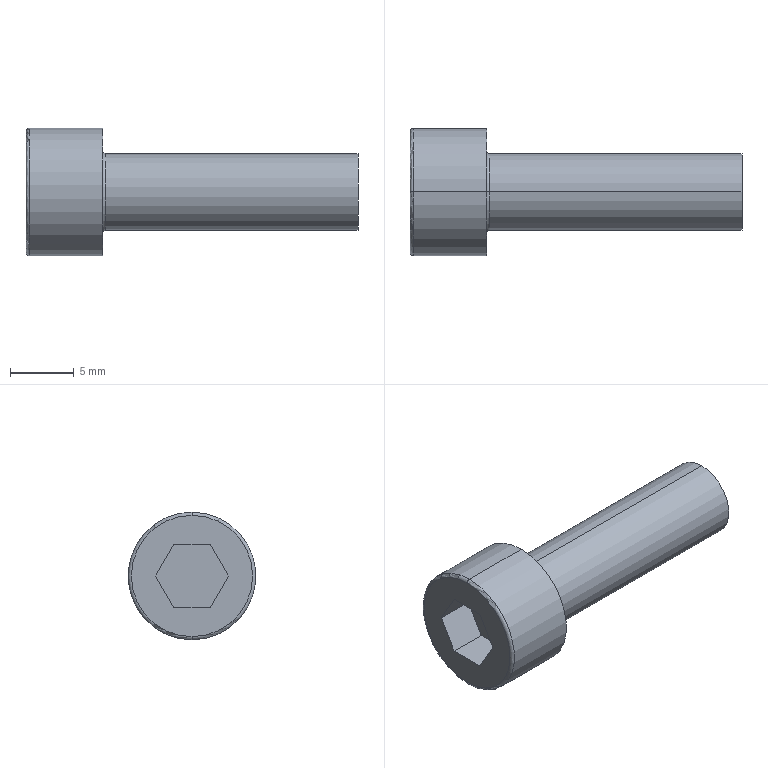Part | SolidWorks | features BlendCut 1, Cut 1, Fillet 1, LPattern 1, RevCut 1, Revolution 1 | 1 solid | 18 faces | box 26 x 10 x 10 mm | volume 972.813 mm3 | plane 10 | torus 4 | cylinder 4 | commonest cylinder face diameters 6 x2 10 x2
STEP:
#1=CARTESIAN_POINT('',(0.25,0.,-5.));
#2=VERTEX_POINT('',#1);
#3=CARTESIAN_POINT('',(0.25,0.,5.));
#4=VERTEX_POINT('',#3);
#5=CARTESIAN_POINT('',(0.25,0.,0.));
#6=DIRECTION('',(1.,0.,0.));
#7=DIRECTION('',(0.,0.,1.));
#8=AXIS2_PLACEMENT_3D('',#5,#6,#7);
#9=CIRCLE('',#8,5.);
#10=EDGE_CURVE('',#2,#4,#9,.T.);
#11=ORIENTED_EDGE('',*,*,#10,.F.);
#12=CARTESIAN_POINT('',(0.,0.,-4.75));
#13=VERTEX_POINT('',#12);
#14=CARTESIAN_POINT('',(0.25,0.,-4.75));
#15=DIRECTION('',(0.,1.,0.));
#16=DIRECTION('',(0.,0.,1.));
#17=AXIS2_PLACEMENT_3D('',#14,#15,#16);
#18=CIRCLE('',#17,0.25);
#19=EDGE_CURVE('',#2,#13,#18,.T.);
#20=ORIENTED_EDGE('',*,*,#19,.T.);
#21=CARTESIAN_POINT('',(0.,0.,4.75));
#22=VERTEX_POINT('',#21);
#23=CARTESIAN_POINT('',(0.,0.,0.));
#24=DIRECTION('',(-1.,0.,0.));
#25=DIRECTION('',(0.,0.,1.));
#26=AXIS2_PLACEMENT_3D('',#23,#24,#25);
#27=CIRCLE('',#26,4.75);
#28=EDGE_CURVE('',#22,#13,#27,.T.);
#29=ORIENTED_EDGE('',*,*,#28,.F.);
#30=CARTESIAN_POINT('',(0.25,0.,4.75));
#31=DIRECTION('',(0.,-1.,0.));
#32=DIRECTION('',(0.,0.,-1.));
#33=AXIS2_PLACEMENT_3D('',#30,#31,#32);
#34=CIRCLE('',#33,0.25);
#35=EDGE_CURVE('',#4,#22,#34,.T.);
#36=ORIENTED_EDGE('',*,*,#35,.F.);
#37=EDGE_LOOP('',(#11,#20,#29,#36));
#38=FACE_OUTER_BOUND('',#37,.T.);
#39=CARTESIAN_POINT('',(0.25,0.,0.));
#40=DIRECTION('',(-1.,0.,0.));
#41=DIRECTION('',(0.,0.,1.));
#42=AXIS2_PLACEMENT_3D('',#39,#40,#41);
#43=TOROIDAL_SURFACE('',#42,4.75,0.25);
#44=ADVANCED_FACE('',(#38),#43,.T.);
#45=CARTESIAN_POINT('',(6.25,0.,-3.));
#46=VERTEX_POINT('',#45);
#47=CARTESIAN_POINT('',(6.25,0.,3.));
#48=VERTEX_POINT('',#47);
#49=CARTESIAN_POINT('',(6.25,0.,0.));
#50=DIRECTION('',(1.,0.,0.));
#51=DIRECTION('',(0.,0.,-1.));
#52=AXIS2_PLACEMENT_3D('',#49,#50,#51);
#53=CIRCLE('',#52,3.);
#54=EDGE_CURVE('',#46,#48,#53,.T.);
#55=ORIENTED_EDGE('',*,*,#54,.T.);
#56=CARTESIAN_POINT('',(26.,0.,3.));
#57=VERTEX_POINT('',#56);
#58=CARTESIAN_POINT('',(0.,0.,3.));
#59=DIRECTION('',(1.,0.,0.));
#60=VECTOR('',#59,1000.);
#61=LINE('',#58,#60);
#62=EDGE_CURVE('',#48,#57,#61,.T.);
#63=ORIENTED_EDGE('',*,*,#62,.T.);
#64=CARTESIAN_POINT('',(26.,0.,-3.));
#65=VERTEX_POINT('',#64);
#66=CARTESIAN_POINT('',(26.,0.,0.));
#67=DIRECTION('',(1.,0.,0.));
#68=DIRECTION('',(0.,0.,-1.));
#69=AXIS2_PLACEMENT_3D('',#66,#67,#68);
#70=CIRCLE('',#69,3.);
#71=EDGE_CURVE('',#65,#57,#70,.T.);
#72=ORIENTED_EDGE('',*,*,#71,.F.);
#73=CARTESIAN_POINT('',(0.,0.,-3.));
#74=DIRECTION('',(1.,0.,0.));
#75=VECTOR('',#74,1000.);
#76=LINE('',#73,#75);
#77=EDGE_CURVE('',#46,#65,#76,.T.);
#78=ORIENTED_EDGE('',*,*,#77,.F.);
#79=EDGE_LOOP('',(#55,#63,#72,#78));
#80=FACE_OUTER_BOUND('',#79,.T.);
#81=CARTESIAN_POINT('',(0.,0.,0.));
#82=DIRECTION('',(1.,0.,0.));
#83=DIRECTION('',(0.,0.,-1.));
#84=AXIS2_PLACEMENT_3D('',#81,#82,#83);
#85=CYLINDRICAL_SURFACE('',#84,3.);
#86=ADVANCED_FACE('',(#80),#85,.T.);
#87=CARTESIAN_POINT('',(6.25,0.,0.));
#88=DIRECTION('',(1.,0.,0.));
#89=DIRECTION('',(0.,0.,-1.));
#90=AXIS2_PLACEMENT_3D('',#87,#88,#89);
#91=CIRCLE('',#90,3.);
#92=EDGE_CURVE('',#48,#46,#91,.T.);
#93=ORIENTED_EDGE('',*,*,#92,.F.);
#94=CARTESIAN_POINT('',(6.,0.,3.25));
#95=VERTEX_POINT('',#94);
#96=CARTESIAN_POINT('',(6.25,0.,3.25));
#97=DIRECTION('',(0.,1.,0.));
#98=DIRECTION('',(0.,0.,1.));
#99=AXIS2_PLACEMENT_3D('',#96,#97,#98);
#100=CIRCLE('',#99,0.25);
#101=EDGE_CURVE('',#48,#95,#100,.T.);
#102=ORIENTED_EDGE('',*,*,#101,.T.);
#103=CARTESIAN_POINT('',(6.,0.,-3.25));
#104=VERTEX_POINT('',#103);
#105=CARTESIAN_POINT('',(6.,0.,0.));
#106=DIRECTION('',(1.,0.,0.));
#107=DIRECTION('',(0.,0.,-1.));
#108=AXIS2_PLACEMENT_3D('',#105,#106,#107);
#109=CIRCLE('',#108,3.25);
#110=EDGE_CURVE('',#95,#104,#109,.T.);
#111=ORIENTED_EDGE('',*,*,#110,.T.);
#112=CARTESIAN_POINT('',(6.25,0.,-3.25));
#113=DIRECTION('',(0.,-1.,0.));
#114=DIRECTION('',(0.,0.,-1.));
#115=AXIS2_PLACEMENT_3D('',#112,#113,#114);
#116=CIRCLE('',#115,0.25);
#117=EDGE_CURVE('',#46,#104,#116,.T.);
#118=ORIENTED_EDGE('',*,*,#117,.F.);
#119=EDGE_LOOP('',(#93,#102,#111,#118));
#120=FACE_OUTER_BOUND('',#119,.T.);
#121=CARTESIAN_POINT('',(6.25,0.,0.));
#122=DIRECTION('',(1.,0.,0.));
#123=DIRECTION('',(0.,0.,-1.));
#124=AXIS2_PLACEMENT_3D('',#121,#122,#123);
#125=TOROIDAL_SURFACE('',#124,3.25,0.25);
#126=ADVANCED_FACE('',(#120),#125,.F.);
#127=ORIENTED_EDGE('',*,*,#10,.T.);
#128=CARTESIAN_POINT('',(6.,0.,5.));
#129=VERTEX_POINT('',#128);
#130=CARTESIAN_POINT('',(0.,0.,5.));
#131=DIRECTION('',(1.,0.,0.));
#132=VECTOR('',#131,1000.);
#133=LINE('',#130,#132);
#134=EDGE_CURVE('',#4,#129,#133,.T.);
#135=ORIENTED_EDGE('',*,*,#134,.T.);
#136=CARTESIAN_POINT('',(6.,0.,-5.));
#137=VERTEX_POINT('',#136);
#138=CARTESIAN_POINT('',(6.,0.,0.));
#139=DIRECTION('',(1.,0.,0.));
#140=DIRECTION('',(0.,0.,-1.));
#141=AXIS2_PLACEMENT_3D('',#138,#139,#140);
#142=CIRCLE('',#141,5.);
#143=EDGE_CURVE('',#137,#129,#142,.T.);
#144=ORIENTED_EDGE('',*,*,#143,.F.);
#145=CARTESIAN_POINT('',(0.,0.,-5.));
#146=DIRECTION('',(1.,0.,0.));
#147=VECTOR('',#146,1000.);
#148=LINE('',#145,#147);
#149=EDGE_CURVE('',#2,#137,#148,.T.);
#150=ORIENTED_EDGE('',*,*,#149,.F.);
#151=EDGE_LOOP('',(#127,#135,#144,#150));
#152=FACE_OUTER_BOUND('',#151,.T.);
#153=CARTESIAN_POINT('',(0.,0.,0.));
#154=DIRECTION('',(1.,0.,0.));
#155=DIRECTION('',(0.,0.,-1.));
#156=AXIS2_PLACEMENT_3D('',#153,#154,#155);
#157=CYLINDRICAL_SURFACE('',#156,5.);
#158=ADVANCED_FACE('',(#152),#157,.T.);
#159=ORIENTED_EDGE('',*,*,#28,.T.);
#160=CARTESIAN_POINT('',(0.,0.,0.));
#161=DIRECTION('',(-1.,0.,0.));
#162=DIRECTION('',(0.,0.,1.));
#163=AXIS2_PLACEMENT_3D('',#160,#161,#162);
#164=CIRCLE('',#163,4.75);
#165=EDGE_CURVE('',#13,#22,#164,.T.);
#166=ORIENTED_EDGE('',*,*,#165,.T.);
#167=EDGE_LOOP('',(#159,#166));
#168=FACE_OUTER_BOUND('',#167,.T.);
#169=CARTESIAN_POINT('',(0.,-2.86,0.));
#170=VERTEX_POINT('',#169);
#171=CARTESIAN_POINT('',(0.,-1.43,2.477));
#172=VERTEX_POINT('',#171);
#173=CARTESIAN_POINT('',(0.,-2.86,0.));
#174=DIRECTION('',(0.,0.5,0.866));
#175=VECTOR('',#174,1000.);
#176=LINE('',#173,#175);
#177=EDGE_CURVE('',#170,#172,#176,.T.);
#178=ORIENTED_EDGE('',*,*,#177,.F.);
#179=CARTESIAN_POINT('',(0.,-1.43,-2.477));
#180=VERTEX_POINT('',#179);
#181=CARTESIAN_POINT('',(0.,-1.43,-2.477));
#182=DIRECTION('',(0.,-0.5,0.866));
#183=VECTOR('',#182,1000.);
#184=LINE('',#181,#183);
#185=EDGE_CURVE('',#180,#170,#184,.T.);
#186=ORIENTED_EDGE('',*,*,#185,.F.);
#187=CARTESIAN_POINT('',(0.,1.43,-2.477));
#188=VERTEX_POINT('',#187);
#189=CARTESIAN_POINT('',(0.,1.43,-2.477));
#190=DIRECTION('',(0.,-1.,0.));
#191=VECTOR('',#190,1000.);
#192=LINE('',#189,#191);
#193=EDGE_CURVE('',#188,#180,#192,.T.);
#194=ORIENTED_EDGE('',*,*,#193,.F.);
#195=CARTESIAN_POINT('',(0.,2.86,0.));
#196=VERTEX_POINT('',#195);
#197=CARTESIAN_POINT('',(0.,2.86,0.));
#198=DIRECTION('',(0.,-0.5,-0.866));
#199=VECTOR('',#198,1000.);
#200=LINE('',#197,#199);
#201=EDGE_CURVE('',#196,#188,#200,.T.);
#202=ORIENTED_EDGE('',*,*,#201,.F.);
#203=CARTESIAN_POINT('',(0.,1.43,2.477));
#204=VERTEX_POINT('',#203);
#205=CARTESIAN_POINT('',(0.,1.43,2.477));
#206=DIRECTION('',(0.,0.5,-0.866));
#207=VECTOR('',#206,1000.);
#208=LINE('',#205,#207);
#209=EDGE_CURVE('',#204,#196,#208,.T.);
#210=ORIENTED_EDGE('',*,*,#209,.F.);
#211=CARTESIAN_POINT('',(0.,-1.43,2.477));
#212=DIRECTION('',(0.,1.,0.));
#213=VECTOR('',#212,1000.);
#214=LINE('',#211,#213);
#215=EDGE_CURVE('',#172,#204,#214,.T.);
#216=ORIENTED_EDGE('',*,*,#215,.F.);
#217=EDGE_LOOP('',(#178,#186,#194,#202,#210,#216));
#218=FACE_BOUND('',#217,.T.);
#219=CARTESIAN_POINT('',(0.,0.,0.));
#220=DIRECTION('',(-1.,0.,0.));
#221=DIRECTION('',(0.,0.,1.));
#222=AXIS2_PLACEMENT_3D('',#219,#220,#221);
#223=PLANE('',#222);
#224=ADVANCED_FACE('',(#168,#218),#223,.T.);
#225=ORIENTED_EDGE('',*,*,#134,.F.);
#226=CARTESIAN_POINT('',(0.25,0.,0.));
#227=DIRECTION('',(1.,0.,0.));
#228=DIRECTION('',(0.,0.,1.));
#229=AXIS2_PLACEMENT_3D('',#226,#227,#228);
#230=CIRCLE('',#229,5.);
#231=EDGE_CURVE('',#4,#2,#230,.T.);
#232=ORIENTED_EDGE('',*,*,#231,.T.);
#233=ORIENTED_EDGE('',*,*,#149,.T.);
#234=CARTESIAN_POINT('',(6.,0.,0.));
#235=DIRECTION('',(1.,0.,0.));
#236=DIRECTION('',(0.,0.,-1.));
#237=AXIS2_PLACEMENT_3D('',#234,#235,#236);
#238=CIRCLE('',#237,5.);
#239=EDGE_CURVE('',#129,#137,#238,.T.);
#240=ORIENTED_EDGE('',*,*,#239,.F.);
#241=EDGE_LOOP('',(#225,#232,#233,#240));
#242=FACE_OUTER_BOUND('',#241,.T.);
#243=CARTESIAN_POINT('',(0.,0.,0.));
#244=DIRECTION('',(1.,0.,0.));
#245=DIRECTION('',(0.,0.,-1.));
#246=AXIS2_PLACEMENT_3D('',#243,#244,#245);
#247=CYLINDRICAL_SURFACE('',#246,5.);
#248=ADVANCED_FACE('',(#242),#247,.T.);
#249=ORIENTED_EDGE('',*,*,#143,.T.);
#250=ORIENTED_EDGE('',*,*,#239,.T.);
#251=EDGE_LOOP('',(#249,#250));
#252=FACE_OUTER_BOUND('',#251,.T.);
#253=CARTESIAN_POINT('',(6.,0.,0.));
#254=DIRECTION('',(1.,0.,0.));
#255=DIRECTION('',(0.,0.,-1.));
#256=AXIS2_PLACEMENT_3D('',#253,#254,#255);
#257=CIRCLE('',#256,3.25);
#258=EDGE_CURVE('',#104,#95,#257,.T.);
#259=ORIENTED_EDGE('',*,*,#258,.F.);
#260=ORIENTED_EDGE('',*,*,#110,.F.);
#261=EDGE_LOOP('',(#259,#260));
#262=FACE_BOUND('',#261,.T.);
#263=CARTESIAN_POINT('',(6.,5.,0.));
#264=DIRECTION('',(1.,0.,0.));
#265=DIRECTION('',(0.,0.,-1.));
#266=AXIS2_PLACEMENT_3D('',#263,#264,#265);
#267=PLANE('',#266);
#268=ADVANCED_FACE('',(#252,#262),#267,.T.);
#269=ORIENTED_EDGE('',*,*,#101,.F.);
#270=ORIENTED_EDGE('',*,*,#54,.F.);
#271=ORIENTED_EDGE('',*,*,#117,.T.);
#272=ORIENTED_EDGE('',*,*,#258,.T.);
#273=EDGE_LOOP('',(#269,#270,#271,#272));
#274=FACE_OUTER_BOUND('',#273,.T.);
#275=CARTESIAN_POINT('',(6.25,0.,0.));
#276=DIRECTION('',(1.,0.,0.));
#277=DIRECTION('',(0.,0.,-1.));
#278=AXIS2_PLACEMENT_3D('',#275,#276,#277);
#279=TOROIDAL_SURFACE('',#278,3.25,0.25);
#280=ADVANCED_FACE('',(#274),#279,.F.);
#281=ORIENTED_EDGE('',*,*,#62,.F.);
#282=ORIENTED_EDGE('',*,*,#92,.T.);
#283=ORIENTED_EDGE('',*,*,#77,.T.);
#284=CARTESIAN_POINT('',(26.,0.,0.));
#285=DIRECTION('',(1.,0.,0.));
#286=DIRECTION('',(0.,0.,-1.));
#287=AXIS2_PLACEMENT_3D('',#284,#285,#286);
#288=CIRCLE('',#287,3.);
#289=EDGE_CURVE('',#57,#65,#288,.T.);
#290=ORIENTED_EDGE('',*,*,#289,.F.);
#291=EDGE_LOOP('',(#281,#282,#283,#290));
#292=FACE_OUTER_BOUND('',#291,.T.);
#293=CARTESIAN_POINT('',(0.,0.,0.));
#294=DIRECTION('',(1.,0.,0.));
#295=DIRECTION('',(0.,0.,-1.));
#296=AXIS2_PLACEMENT_3D('',#293,#294,#295);
#297=CYLINDRICAL_SURFACE('',#296,3.);
#298=ADVANCED_FACE('',(#292),#297,.T.);
#299=ORIENTED_EDGE('',*,*,#71,.T.);
#300=ORIENTED_EDGE('',*,*,#289,.T.);
#301=EDGE_LOOP('',(#299,#300));
#302=FACE_OUTER_BOUND('',#301,.T.);
#303=CARTESIAN_POINT('',(26.,3.,0.));
#304=DIRECTION('',(1.,0.,0.));
#305=DIRECTION('',(0.,0.,-1.));
#306=AXIS2_PLACEMENT_3D('',#303,#304,#305);
#307=PLANE('',#306);
#308=ADVANCED_FACE('',(#302),#307,.T.);
#309=ORIENTED_EDGE('',*,*,#177,.T.);
#310=CARTESIAN_POINT('',(3.,-1.43,2.477));
#311=VERTEX_POINT('',#310);
#312=CARTESIAN_POINT('',(3.,-1.43,2.477));
#313=DIRECTION('',(-1.,0.,0.));
#314=VECTOR('',#313,1000.);
#315=LINE('',#312,#314);
#316=EDGE_CURVE('',#311,#172,#315,.T.);
#317=ORIENTED_EDGE('',*,*,#316,.F.);
#318=CARTESIAN_POINT('',(3.,-2.86,0.));
#319=VERTEX_POINT('',#318);
#320=CARTESIAN_POINT('',(3.,-2.86,0.));
#321=DIRECTION('',(0.,0.5,0.866));
#322=VECTOR('',#321,1000.);
#323=LINE('',#320,#322);
#324=EDGE_CURVE('',#319,#311,#323,.T.);
#325=ORIENTED_EDGE('',*,*,#324,.F.);
#326=CARTESIAN_POINT('',(3.,-2.86,0.));
#327=DIRECTION('',(-1.,0.,0.));
#328=VECTOR('',#327,1000.);
#329=LINE('',#326,#328);
#330=EDGE_CURVE('',#319,#170,#329,.T.);
#331=ORIENTED_EDGE('',*,*,#330,.T.);
#332=EDGE_LOOP('',(#309,#317,#325,#331));
#333=FACE_OUTER_BOUND('',#332,.T.);
#334=CARTESIAN_POINT('',(3.,-2.86,0.));
#335=DIRECTION('',(0.,-0.866,0.5));
#336=DIRECTION('',(0.,-0.5,-0.866));
#337=AXIS2_PLACEMENT_3D('',#334,#335,#336);
#338=PLANE('',#337);
#339=ADVANCED_FACE('',(#333),#338,.F.);
#340=ORIENTED_EDGE('',*,*,#185,.T.);
#341=ORIENTED_EDGE('',*,*,#330,.F.);
#342=CARTESIAN_POINT('',(3.,-1.43,-2.477));
#343=VERTEX_POINT('',#342);
#344=CARTESIAN_POINT('',(3.,-1.43,-2.477));
#345=DIRECTION('',(0.,-0.5,0.866));
#346=VECTOR('',#345,1000.);
#347=LINE('',#344,#346);
#348=EDGE_CURVE('',#343,#319,#347,.T.);
#349=ORIENTED_EDGE('',*,*,#348,.F.);
#350=CARTESIAN_POINT('',(3.,-1.43,-2.477));
#351=DIRECTION('',(-1.,0.,0.));
#352=VECTOR('',#351,1000.);
#353=LINE('',#350,#352);
#354=EDGE_CURVE('',#343,#180,#353,.T.);
#355=ORIENTED_EDGE('',*,*,#354,.T.);
#356=EDGE_LOOP('',(#340,#341,#349,#355));
#357=FACE_OUTER_BOUND('',#356,.T.);
#358=CARTESIAN_POINT('',(3.,-1.43,-2.477));
#359=DIRECTION('',(0.,-0.866,-0.5));
#360=DIRECTION('',(0.,0.5,-0.866));
#361=AXIS2_PLACEMENT_3D('',#358,#359,#360);
#362=PLANE('',#361);
#363=ADVANCED_FACE('',(#357),#362,.F.);
#364=ORIENTED_EDGE('',*,*,#193,.T.);
#365=ORIENTED_EDGE('',*,*,#354,.F.);
#366=CARTESIAN_POINT('',(3.,1.43,-2.477));
#367=VERTEX_POINT('',#366);
#368=CARTESIAN_POINT('',(3.,1.43,-2.477));
#369=DIRECTION('',(0.,-1.,0.));
#370=VECTOR('',#369,1000.);
#371=LINE('',#368,#370);
#372=EDGE_CURVE('',#367,#343,#371,.T.);
#373=ORIENTED_EDGE('',*,*,#372,.F.);
#374=CARTESIAN_POINT('',(3.,1.43,-2.477));
#375=DIRECTION('',(-1.,0.,0.));
#376=VECTOR('',#375,1000.);
#377=LINE('',#374,#376);
#378=EDGE_CURVE('',#367,#188,#377,.T.);
#379=ORIENTED_EDGE('',*,*,#378,.T.);
#380=EDGE_LOOP('',(#364,#365,#373,#379));
#381=FACE_OUTER_BOUND('',#380,.T.);
#382=CARTESIAN_POINT('',(3.,1.43,-2.477));
#383=DIRECTION('',(0.,0.,-1.));
#384=DIRECTION('',(-1.,0.,0.));
#385=AXIS2_PLACEMENT_3D('',#382,#383,#384);
#386=PLANE('',#385);
#387=ADVANCED_FACE('',(#381),#386,.F.);
#388=ORIENTED_EDGE('',*,*,#201,.T.);
#389=ORIENTED_EDGE('',*,*,#378,.F.);
#390=CARTESIAN_POINT('',(3.,2.86,0.));
#391=VERTEX_POINT('',#390);
#392=CARTESIAN_POINT('',(3.,2.86,0.));
#393=DIRECTION('',(0.,-0.5,-0.866));
#394=VECTOR('',#393,1000.);
#395=LINE('',#392,#394);
#396=EDGE_CURVE('',#391,#367,#395,.T.);
#397=ORIENTED_EDGE('',*,*,#396,.F.);
#398=CARTESIAN_POINT('',(3.,2.86,0.));
#399=DIRECTION('',(-1.,0.,0.));
#400=VECTOR('',#399,1000.);
#401=LINE('',#398,#400);
#402=EDGE_CURVE('',#391,#196,#401,.T.);
#403=ORIENTED_EDGE('',*,*,#402,.T.);
#404=EDGE_LOOP('',(#388,#389,#397,#403));
#405=FACE_OUTER_BOUND('',#404,.T.);
#406=CARTESIAN_POINT('',(3.,2.86,0.));
#407=DIRECTION('',(0.,0.866,-0.5));
#408=DIRECTION('',(0.,0.5,0.866));
#409=AXIS2_PLACEMENT_3D('',#406,#407,#408);
#410=PLANE('',#409);
#411=ADVANCED_FACE('',(#405),#410,.F.);
#412=ORIENTED_EDGE('',*,*,#209,.T.);
#413=ORIENTED_EDGE('',*,*,#402,.F.);
#414=CARTESIAN_POINT('',(3.,1.43,2.477));
#415=VERTEX_POINT('',#414);
#416=CARTESIAN_POINT('',(3.,1.43,2.477));
#417=DIRECTION('',(0.,0.5,-0.866));
#418=VECTOR('',#417,1000.);
#419=LINE('',#416,#418);
#420=EDGE_CURVE('',#415,#391,#419,.T.);
#421=ORIENTED_EDGE('',*,*,#420,.F.);
#422=CARTESIAN_POINT('',(3.,1.43,2.477));
#423=DIRECTION('',(-1.,0.,0.));
#424=VECTOR('',#423,1000.);
#425=LINE('',#422,#424);
#426=EDGE_CURVE('',#415,#204,#425,.T.);
#427=ORIENTED_EDGE('',*,*,#426,.T.);
#428=EDGE_LOOP('',(#412,#413,#421,#427));
#429=FACE_OUTER_BOUND('',#428,.T.);
#430=CARTESIAN_POINT('',(3.,1.43,2.477));
#431=DIRECTION('',(0.,0.866,0.5));
#432=DIRECTION('',(0.,-0.5,0.866));
#433=AXIS2_PLACEMENT_3D('',#430,#431,#432);
#434=PLANE('',#433);
#435=ADVANCED_FACE('',(#429),#434,.F.);
#436=ORIENTED_EDGE('',*,*,#215,.T.);
#437=ORIENTED_EDGE('',*,*,#426,.F.);
#438=CARTESIAN_POINT('',(3.,-1.43,2.477));
#439=DIRECTION('',(0.,1.,0.));
#440=VECTOR('',#439,1000.);
#441=LINE('',#438,#440);
#442=EDGE_CURVE('',#311,#415,#441,.T.);
#443=ORIENTED_EDGE('',*,*,#442,.F.);
#444=ORIENTED_EDGE('',*,*,#316,.T.);
#445=EDGE_LOOP('',(#436,#437,#443,#444));
#446=FACE_OUTER_BOUND('',#445,.T.);
#447=CARTESIAN_POINT('',(3.,-1.43,2.477));
#448=DIRECTION('',(0.,0.,1.));
#449=DIRECTION('',(0.,-1.,0.));
#450=AXIS2_PLACEMENT_3D('',#447,#448,#449);
#451=PLANE('',#450);
#452=ADVANCED_FACE('',(#446),#451,.F.);
#453=ORIENTED_EDGE('',*,*,#324,.T.);
#454=ORIENTED_EDGE('',*,*,#442,.T.);
#455=ORIENTED_EDGE('',*,*,#420,.T.);
#456=ORIENTED_EDGE('',*,*,#396,.T.);
#457=ORIENTED_EDGE('',*,*,#372,.T.);
#458=ORIENTED_EDGE('',*,*,#348,.T.);
#459=EDGE_LOOP('',(#453,#454,#455,#456,#457,#458));
#460=FACE_OUTER_BOUND('',#459,.T.);
#461=CARTESIAN_POINT('',(3.,-1.43,2.477));
#462=DIRECTION('',(-1.,0.,0.));
#463=DIRECTION('',(0.,0.,1.));
#464=AXIS2_PLACEMENT_3D('',#461,#462,#463);
#465=PLANE('',#464);
#466=ADVANCED_FACE('',(#460),#465,.T.);
#467=ORIENTED_EDGE('',*,*,#19,.F.);
#468=ORIENTED_EDGE('',*,*,#231,.F.);
#469=ORIENTED_EDGE('',*,*,#35,.T.);
#470=ORIENTED_EDGE('',*,*,#165,.F.);
#471=EDGE_LOOP('',(#467,#468,#469,#470));
#472=FACE_OUTER_BOUND('',#471,.T.);
#473=CARTESIAN_POINT('',(0.25,0.,0.));
#474=DIRECTION('',(-1.,0.,0.));
#475=DIRECTION('',(0.,0.,1.));
#476=AXIS2_PLACEMENT_3D('',#473,#474,#475);
#477=TOROIDAL_SURFACE('',#476,4.75,0.25);
#478=ADVANCED_FACE('',(#472),#477,.T.);
#479=CLOSED_SHELL('',(#44,#86,#126,#158,#224,#248,#268,#280,#298,#308,#339,#363,#387,#411,#435,#452,#466,#478));
#480=MANIFOLD_SOLID_BREP('',#479);
#481=CARTESIAN_POINT('',(0.,0.,0.));
#482=DIRECTION('',(0.,0.,1.));
#483=DIRECTION('',(1.,0.,0.));
#484=AXIS2_PLACEMENT_3D('',#481,#482,#483);
#485=(LENGTH_UNIT()NAMED_UNIT(*)SI_UNIT(.MILLI.,.METRE.));
#486=UNCERTAINTY_MEASURE_WITH_UNIT(LENGTH_MEASURE(0.00001),#485,'','');
#487=(NAMED_UNIT(*)PLANE_ANGLE_UNIT()SI_UNIT($,.RADIAN.));
#488=(NAMED_UNIT(*)SI_UNIT($,.STERADIAN.)SOLID_ANGLE_UNIT());
#489=(GEOMETRIC_REPRESENTATION_CONTEXT(3)GLOBAL_UNCERTAINTY_ASSIGNED_CONTEXT((#486))GLOBAL_UNIT_ASSIGNED_CONTEXT((#485,#487,#488))REPRESENTATION_CONTEXT('',''));
#490=ADVANCED_BREP_SHAPE_REPRESENTATION('',(#480,#484),#489);